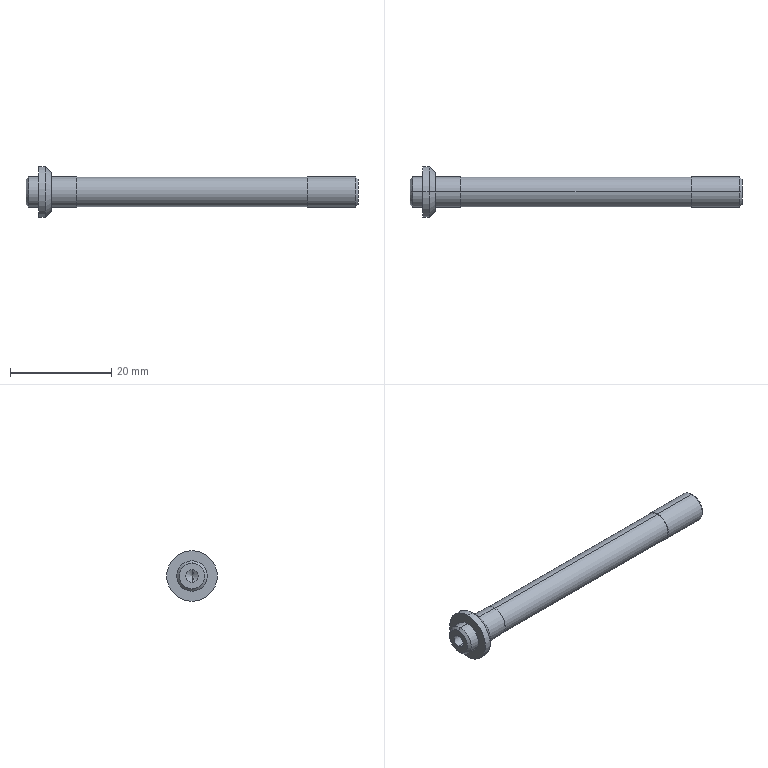Part | SolidWorks | features Chamfer 2, HoleWzd 1, Revolution 1 | 1 solid | 26 faces | box 65.5 x 10 x 10 mm | volume 1830 mm3 | cylinder 12 | cone 8 | plane 6 | commonest cylinder face diameters 6 x6 2.5 x2 5.8 x2 10 x2
STEP:
#1=CARTESIAN_POINT('',(65.5,0.,-2.5));
#2=VERTEX_POINT('',#1);
#3=CARTESIAN_POINT('',(65.5,0.,2.5));
#4=VERTEX_POINT('',#3);
#5=CARTESIAN_POINT('',(65.5,0.,0.));
#6=DIRECTION('',(1.,0.,0.));
#7=DIRECTION('',(0.,0.,1.));
#8=AXIS2_PLACEMENT_3D('',#5,#6,#7);
#9=CIRCLE('',#8,2.5);
#10=EDGE_CURVE('',#2,#4,#9,.T.);
#11=ORIENTED_EDGE('',*,*,#10,.F.);
#12=CARTESIAN_POINT('',(65.,0.,-3.));
#13=VERTEX_POINT('',#12);
#14=CARTESIAN_POINT('',(65.,0.,-3.));
#15=DIRECTION('',(-0.7071,0.,-0.7071));
#16=VECTOR('',#15,1000.);
#17=LINE('',#14,#16);
#18=EDGE_CURVE('',#2,#13,#17,.T.);
#19=ORIENTED_EDGE('',*,*,#18,.T.);
#20=CARTESIAN_POINT('',(65.,0.,3.));
#21=VERTEX_POINT('',#20);
#22=CARTESIAN_POINT('',(65.,0.,0.));
#23=DIRECTION('',(-1.,0.,0.));
#24=DIRECTION('',(0.,0.,1.));
#25=AXIS2_PLACEMENT_3D('',#22,#23,#24);
#26=CIRCLE('',#25,3.);
#27=EDGE_CURVE('',#21,#13,#26,.T.);
#28=ORIENTED_EDGE('',*,*,#27,.F.);
#29=CARTESIAN_POINT('',(65.,0.,3.));
#30=DIRECTION('',(-0.7071,0.,0.7071));
#31=VECTOR('',#30,1000.);
#32=LINE('',#29,#31);
#33=EDGE_CURVE('',#4,#21,#32,.T.);
#34=ORIENTED_EDGE('',*,*,#33,.F.);
#35=EDGE_LOOP('',(#11,#19,#28,#34));
#36=FACE_OUTER_BOUND('',#35,.T.);
#37=CARTESIAN_POINT('',(65.,0.,0.));
#38=DIRECTION('',(-1.,0.,0.));
#39=DIRECTION('',(0.,0.,1.));
#40=AXIS2_PLACEMENT_3D('',#37,#38,#39);
#41=CONICAL_SURFACE('',#40,3.,0.7854);
#42=ADVANCED_FACE('',(#36),#41,.T.);
#43=CARTESIAN_POINT('',(0.,0.,2.5));
#44=VERTEX_POINT('',#43);
#45=CARTESIAN_POINT('',(0.,0.,-2.5));
#46=VERTEX_POINT('',#45);
#47=CARTESIAN_POINT('',(0.,0.,0.));
#48=DIRECTION('',(-1.,0.,0.));
#49=DIRECTION('',(0.,0.,-1.));
#50=AXIS2_PLACEMENT_3D('',#47,#48,#49);
#51=CIRCLE('',#50,2.5);
#52=EDGE_CURVE('',#44,#46,#51,.T.);
#53=ORIENTED_EDGE('',*,*,#52,.F.);
#54=CARTESIAN_POINT('',(0.5,0.,3.));
#55=VERTEX_POINT('',#54);
#56=CARTESIAN_POINT('',(0.,0.,2.5));
#57=DIRECTION('',(0.7071,0.,0.7071));
#58=VECTOR('',#57,1000.);
#59=LINE('',#56,#58);
#60=EDGE_CURVE('',#44,#55,#59,.T.);
#61=ORIENTED_EDGE('',*,*,#60,.T.);
#62=CARTESIAN_POINT('',(0.5,0.,-3.));
#63=VERTEX_POINT('',#62);
#64=CARTESIAN_POINT('',(0.5,0.,0.));
#65=DIRECTION('',(1.,0.,0.));
#66=DIRECTION('',(0.,0.,-1.));
#67=AXIS2_PLACEMENT_3D('',#64,#65,#66);
#68=CIRCLE('',#67,3.);
#69=EDGE_CURVE('',#63,#55,#68,.T.);
#70=ORIENTED_EDGE('',*,*,#69,.F.);
#71=CARTESIAN_POINT('',(0.,0.,-2.5));
#72=DIRECTION('',(0.7071,0.,-0.7071));
#73=VECTOR('',#72,1000.);
#74=LINE('',#71,#73);
#75=EDGE_CURVE('',#46,#63,#74,.T.);
#76=ORIENTED_EDGE('',*,*,#75,.F.);
#77=EDGE_LOOP('',(#53,#61,#70,#76));
#78=FACE_OUTER_BOUND('',#77,.T.);
#79=CARTESIAN_POINT('',(0.,0.,0.));
#80=DIRECTION('',(1.,0.,0.));
#81=DIRECTION('',(0.,0.,-1.));
#82=AXIS2_PLACEMENT_3D('',#79,#80,#81);
#83=CONICAL_SURFACE('',#82,2.5,0.7854);
#84=ADVANCED_FACE('',(#78),#83,.T.);
#85=CARTESIAN_POINT('',(7.5,0.,-1.25));
#86=VERTEX_POINT('',#85);
#87=CARTESIAN_POINT('',(7.5,0.,1.25));
#88=VERTEX_POINT('',#87);
#89=CARTESIAN_POINT('',(7.5,0.,0.));
#90=DIRECTION('',(-1.,0.,0.));
#91=DIRECTION('',(0.,0.,1.));
#92=AXIS2_PLACEMENT_3D('',#89,#90,#91);
#93=CIRCLE('',#92,1.25);
#94=EDGE_CURVE('',#86,#88,#93,.T.);
#95=ORIENTED_EDGE('',*,*,#94,.F.);
#96=CARTESIAN_POINT('',(0.,0.,-1.25));
#97=VERTEX_POINT('',#96);
#98=CARTESIAN_POINT('',(0.,0.,-1.25));
#99=DIRECTION('',(-1.,0.,0.));
#100=VECTOR('',#99,1000.);
#101=LINE('',#98,#100);
#102=EDGE_CURVE('',#86,#97,#101,.T.);
#103=ORIENTED_EDGE('',*,*,#102,.T.);
#104=CARTESIAN_POINT('',(0.,0.,1.25));
#105=VERTEX_POINT('',#104);
#106=CARTESIAN_POINT('',(0.,0.,0.));
#107=DIRECTION('',(-1.,0.,0.));
#108=DIRECTION('',(0.,0.,1.));
#109=AXIS2_PLACEMENT_3D('',#106,#107,#108);
#110=CIRCLE('',#109,1.25);
#111=EDGE_CURVE('',#97,#105,#110,.T.);
#112=ORIENTED_EDGE('',*,*,#111,.T.);
#113=CARTESIAN_POINT('',(0.,0.,1.25));
#114=DIRECTION('',(-1.,0.,0.));
#115=VECTOR('',#114,1000.);
#116=LINE('',#113,#115);
#117=EDGE_CURVE('',#88,#105,#116,.T.);
#118=ORIENTED_EDGE('',*,*,#117,.F.);
#119=EDGE_LOOP('',(#95,#103,#112,#118));
#120=FACE_OUTER_BOUND('',#119,.T.);
#121=CARTESIAN_POINT('',(0.,0.,0.));
#122=DIRECTION('',(-1.,0.,0.));
#123=DIRECTION('',(0.,0.,1.));
#124=AXIS2_PLACEMENT_3D('',#121,#122,#123);
#125=CYLINDRICAL_SURFACE('',#124,1.25);
#126=ADVANCED_FACE('',(#120),#125,.F.);
#127=CARTESIAN_POINT('',(8.251,0.,0.));
#128=VERTEX_POINT('',#127);
#129=CARTESIAN_POINT('',(7.5,0.,1.25));
#130=DIRECTION('',(-0.515,0.,0.8572));
#131=VECTOR('',#130,1000.);
#132=LINE('',#129,#131);
#133=EDGE_CURVE('',#128,#88,#132,.T.);
#134=ORIENTED_EDGE('',*,*,#133,.F.);
#135=CARTESIAN_POINT('',(7.5,0.,-1.25));
#136=DIRECTION('',(-0.515,0.,-0.8572));
#137=VECTOR('',#136,1000.);
#138=LINE('',#135,#137);
#139=EDGE_CURVE('',#128,#86,#138,.T.);
#140=ORIENTED_EDGE('',*,*,#139,.T.);
#141=ORIENTED_EDGE('',*,*,#94,.T.);
#142=EDGE_LOOP('',(#134,#140,#141));
#143=FACE_OUTER_BOUND('',#142,.T.);
#144=CARTESIAN_POINT('',(7.5,0.,0.));
#145=DIRECTION('',(-1.,0.,0.));
#146=DIRECTION('',(0.,0.,1.));
#147=AXIS2_PLACEMENT_3D('',#144,#145,#146);
#148=CONICAL_SURFACE('',#147,1.25,1.03);
#149=ADVANCED_FACE('',(#143),#148,.F.);
#150=CARTESIAN_POINT('',(5.,0.,-3.8));
#151=VERTEX_POINT('',#150);
#152=CARTESIAN_POINT('',(5.,0.,3.8));
#153=VERTEX_POINT('',#152);
#154=CARTESIAN_POINT('',(5.,0.,0.));
#155=DIRECTION('',(1.,0.,0.));
#156=DIRECTION('',(0.,0.,1.));
#157=AXIS2_PLACEMENT_3D('',#154,#155,#156);
#158=CIRCLE('',#157,3.8);
#159=EDGE_CURVE('',#151,#153,#158,.T.);
#160=ORIENTED_EDGE('',*,*,#159,.F.);
#161=CARTESIAN_POINT('',(3.8,0.,-5.));
#162=VERTEX_POINT('',#161);
#163=CARTESIAN_POINT('',(3.8,0.,-5.));
#164=DIRECTION('',(-0.7071,0.,-0.7071));
#165=VECTOR('',#164,1000.);
#166=LINE('',#163,#165);
#167=EDGE_CURVE('',#151,#162,#166,.T.);
#168=ORIENTED_EDGE('',*,*,#167,.T.);
#169=CARTESIAN_POINT('',(3.8,0.,5.));
#170=VERTEX_POINT('',#169);
#171=CARTESIAN_POINT('',(3.8,0.,0.));
#172=DIRECTION('',(-1.,0.,0.));
#173=DIRECTION('',(0.,0.,1.));
#174=AXIS2_PLACEMENT_3D('',#171,#172,#173);
#175=CIRCLE('',#174,5.);
#176=EDGE_CURVE('',#170,#162,#175,.T.);
#177=ORIENTED_EDGE('',*,*,#176,.F.);
#178=CARTESIAN_POINT('',(3.8,0.,5.));
#179=DIRECTION('',(-0.7071,0.,0.7071));
#180=VECTOR('',#179,1000.);
#181=LINE('',#178,#180);
#182=EDGE_CURVE('',#153,#170,#181,.T.);
#183=ORIENTED_EDGE('',*,*,#182,.F.);
#184=EDGE_LOOP('',(#160,#168,#177,#183));
#185=FACE_OUTER_BOUND('',#184,.T.);
#186=CARTESIAN_POINT('',(3.8,0.,0.));
#187=DIRECTION('',(-1.,0.,0.));
#188=DIRECTION('',(0.,0.,1.));
#189=AXIS2_PLACEMENT_3D('',#186,#187,#188);
#190=CONICAL_SURFACE('',#189,5.,0.7854);
#191=ADVANCED_FACE('',(#185),#190,.T.);
#192=ORIENTED_EDGE('',*,*,#27,.T.);
#193=CARTESIAN_POINT('',(55.5,0.,-3.));
#194=VERTEX_POINT('',#193);
#195=CARTESIAN_POINT('',(0.,0.,-3.));
#196=DIRECTION('',(-1.,0.,0.));
#197=VECTOR('',#196,1000.);
#198=LINE('',#195,#197);
#199=EDGE_CURVE('',#13,#194,#198,.T.);
#200=ORIENTED_EDGE('',*,*,#199,.T.);
#201=CARTESIAN_POINT('',(55.5,0.,3.));
#202=VERTEX_POINT('',#201);
#203=CARTESIAN_POINT('',(55.5,0.,0.));
#204=DIRECTION('',(-1.,0.,0.));
#205=DIRECTION('',(0.,0.,1.));
#206=AXIS2_PLACEMENT_3D('',#203,#204,#205);
#207=CIRCLE('',#206,3.);
#208=EDGE_CURVE('',#202,#194,#207,.T.);
#209=ORIENTED_EDGE('',*,*,#208,.F.);
#210=CARTESIAN_POINT('',(0.,0.,3.));
#211=DIRECTION('',(-1.,0.,0.));
#212=VECTOR('',#211,1000.);
#213=LINE('',#210,#212);
#214=EDGE_CURVE('',#21,#202,#213,.T.);
#215=ORIENTED_EDGE('',*,*,#214,.F.);
#216=EDGE_LOOP('',(#192,#200,#209,#215));
#217=FACE_OUTER_BOUND('',#216,.T.);
#218=CARTESIAN_POINT('',(0.,0.,0.));
#219=DIRECTION('',(-1.,0.,0.));
#220=DIRECTION('',(0.,0.,1.));
#221=AXIS2_PLACEMENT_3D('',#218,#219,#220);
#222=CYLINDRICAL_SURFACE('',#221,3.);
#223=ADVANCED_FACE('',(#217),#222,.T.);
#224=CARTESIAN_POINT('',(55.5,0.,2.9));
#225=VERTEX_POINT('',#224);
#226=CARTESIAN_POINT('',(55.5,0.,-2.9));
#227=VERTEX_POINT('',#226);
#228=CARTESIAN_POINT('',(55.5,0.,0.));
#229=DIRECTION('',(-1.,0.,0.));
#230=DIRECTION('',(0.,0.,1.));
#231=AXIS2_PLACEMENT_3D('',#228,#229,#230);
#232=CIRCLE('',#231,2.9);
#233=EDGE_CURVE('',#225,#227,#232,.T.);
#234=ORIENTED_EDGE('',*,*,#233,.T.);
#235=CARTESIAN_POINT('',(10.,0.,-2.9));
#236=VERTEX_POINT('',#235);
#237=CARTESIAN_POINT('',(0.,0.,-2.9));
#238=DIRECTION('',(-1.,0.,0.));
#239=VECTOR('',#238,1000.);
#240=LINE('',#237,#239);
#241=EDGE_CURVE('',#227,#236,#240,.T.);
#242=ORIENTED_EDGE('',*,*,#241,.T.);
#243=CARTESIAN_POINT('',(10.,0.,2.9));
#244=VERTEX_POINT('',#243);
#245=CARTESIAN_POINT('',(10.,0.,0.));
#246=DIRECTION('',(-1.,0.,0.));
#247=DIRECTION('',(0.,0.,1.));
#248=AXIS2_PLACEMENT_3D('',#245,#246,#247);
#249=CIRCLE('',#248,2.9);
#250=EDGE_CURVE('',#244,#236,#249,.T.);
#251=ORIENTED_EDGE('',*,*,#250,.F.);
#252=CARTESIAN_POINT('',(0.,0.,2.9));
#253=DIRECTION('',(-1.,0.,0.));
#254=VECTOR('',#253,1000.);
#255=LINE('',#252,#254);
#256=EDGE_CURVE('',#225,#244,#255,.T.);
#257=ORIENTED_EDGE('',*,*,#256,.F.);
#258=EDGE_LOOP('',(#234,#242,#251,#257));
#259=FACE_OUTER_BOUND('',#258,.T.);
#260=CARTESIAN_POINT('',(0.,0.,0.));
#261=DIRECTION('',(-1.,0.,0.));
#262=DIRECTION('',(0.,0.,1.));
#263=AXIS2_PLACEMENT_3D('',#260,#261,#262);
#264=CYLINDRICAL_SURFACE('',#263,2.9);
#265=ADVANCED_FACE('',(#259),#264,.T.);
#266=CARTESIAN_POINT('',(10.,0.,3.));
#267=VERTEX_POINT('',#266);
#268=CARTESIAN_POINT('',(10.,0.,-3.));
#269=VERTEX_POINT('',#268);
#270=CARTESIAN_POINT('',(10.,0.,0.));
#271=DIRECTION('',(-1.,0.,0.));
#272=DIRECTION('',(0.,0.,1.));
#273=AXIS2_PLACEMENT_3D('',#270,#271,#272);
#274=CIRCLE('',#273,3.);
#275=EDGE_CURVE('',#267,#269,#274,.T.);
#276=ORIENTED_EDGE('',*,*,#275,.T.);
#277=CARTESIAN_POINT('',(5.,0.,-3.));
#278=VERTEX_POINT('',#277);
#279=CARTESIAN_POINT('',(0.,0.,-3.));
#280=DIRECTION('',(-1.,0.,0.));
#281=VECTOR('',#280,1000.);
#282=LINE('',#279,#281);
#283=EDGE_CURVE('',#269,#278,#282,.T.);
#284=ORIENTED_EDGE('',*,*,#283,.T.);
#285=CARTESIAN_POINT('',(5.,0.,3.));
#286=VERTEX_POINT('',#285);
#287=CARTESIAN_POINT('',(5.,0.,0.));
#288=DIRECTION('',(-1.,0.,0.));
#289=DIRECTION('',(0.,0.,1.));
#290=AXIS2_PLACEMENT_3D('',#287,#288,#289);
#291=CIRCLE('',#290,3.);
#292=EDGE_CURVE('',#286,#278,#291,.T.);
#293=ORIENTED_EDGE('',*,*,#292,.F.);
#294=CARTESIAN_POINT('',(0.,0.,3.));
#295=DIRECTION('',(-1.,0.,0.));
#296=VECTOR('',#295,1000.);
#297=LINE('',#294,#296);
#298=EDGE_CURVE('',#267,#286,#297,.T.);
#299=ORIENTED_EDGE('',*,*,#298,.F.);
#300=EDGE_LOOP('',(#276,#284,#293,#299));
#301=FACE_OUTER_BOUND('',#300,.T.);
#302=CARTESIAN_POINT('',(0.,0.,0.));
#303=DIRECTION('',(-1.,0.,0.));
#304=DIRECTION('',(0.,0.,1.));
#305=AXIS2_PLACEMENT_3D('',#302,#303,#304);
#306=CYLINDRICAL_SURFACE('',#305,3.);
#307=ADVANCED_FACE('',(#301),#306,.T.);
#308=ORIENTED_EDGE('',*,*,#176,.T.);
#309=CARTESIAN_POINT('',(2.5,0.,-5.));
#310=VERTEX_POINT('',#309);
#311=CARTESIAN_POINT('',(0.,0.,-5.));
#312=DIRECTION('',(-1.,0.,0.));
#313=VECTOR('',#312,1000.);
#314=LINE('',#311,#313);
#315=EDGE_CURVE('',#162,#310,#314,.T.);
#316=ORIENTED_EDGE('',*,*,#315,.T.);
#317=CARTESIAN_POINT('',(2.5,0.,5.));
#318=VERTEX_POINT('',#317);
#319=CARTESIAN_POINT('',(2.5,0.,0.));
#320=DIRECTION('',(-1.,0.,0.));
#321=DIRECTION('',(0.,0.,1.));
#322=AXIS2_PLACEMENT_3D('',#319,#320,#321);
#323=CIRCLE('',#322,5.);
#324=EDGE_CURVE('',#318,#310,#323,.T.);
#325=ORIENTED_EDGE('',*,*,#324,.F.);
#326=CARTESIAN_POINT('',(0.,0.,5.));
#327=DIRECTION('',(-1.,0.,0.));
#328=VECTOR('',#327,1000.);
#329=LINE('',#326,#328);
#330=EDGE_CURVE('',#170,#318,#329,.T.);
#331=ORIENTED_EDGE('',*,*,#330,.F.);
#332=EDGE_LOOP('',(#308,#316,#325,#331));
#333=FACE_OUTER_BOUND('',#332,.T.);
#334=CARTESIAN_POINT('',(0.,0.,0.));
#335=DIRECTION('',(-1.,0.,0.));
#336=DIRECTION('',(0.,0.,1.));
#337=AXIS2_PLACEMENT_3D('',#334,#335,#336);
#338=CYLINDRICAL_SURFACE('',#337,5.);
#339=ADVANCED_FACE('',(#333),#338,.T.);
#340=CARTESIAN_POINT('',(2.5,0.,3.));
#341=VERTEX_POINT('',#340);
#342=CARTESIAN_POINT('',(2.5,0.,-3.));
#343=VERTEX_POINT('',#342);
#344=CARTESIAN_POINT('',(2.5,0.,0.));
#345=DIRECTION('',(-1.,0.,0.));
#346=DIRECTION('',(0.,0.,1.));
#347=AXIS2_PLACEMENT_3D('',#344,#345,#346);
#348=CIRCLE('',#347,3.);
#349=EDGE_CURVE('',#341,#343,#348,.T.);
#350=ORIENTED_EDGE('',*,*,#349,.T.);
#351=CARTESIAN_POINT('',(0.,0.,-3.));
#352=DIRECTION('',(-1.,0.,0.));
#353=VECTOR('',#352,1000.);
#354=LINE('',#351,#353);
#355=EDGE_CURVE('',#343,#63,#354,.T.);
#356=ORIENTED_EDGE('',*,*,#355,.T.);
#357=ORIENTED_EDGE('',*,*,#69,.T.);
#358=CARTESIAN_POINT('',(0.,0.,3.));
#359=DIRECTION('',(-1.,0.,0.));
#360=VECTOR('',#359,1000.);
#361=LINE('',#358,#360);
#362=EDGE_CURVE('',#341,#55,#361,.T.);
#363=ORIENTED_EDGE('',*,*,#362,.F.);
#364=EDGE_LOOP('',(#350,#356,#357,#363));
#365=FACE_OUTER_BOUND('',#364,.T.);
#366=CARTESIAN_POINT('',(0.,0.,0.));
#367=DIRECTION('',(-1.,0.,0.));
#368=DIRECTION('',(0.,0.,1.));
#369=AXIS2_PLACEMENT_3D('',#366,#367,#368);
#370=CYLINDRICAL_SURFACE('',#369,3.);
#371=ADVANCED_FACE('',(#365),#370,.T.);
#372=CARTESIAN_POINT('',(0.,0.,0.));
#373=DIRECTION('',(-1.,0.,0.));
#374=DIRECTION('',(0.,0.,-1.));
#375=AXIS2_PLACEMENT_3D('',#372,#373,#374);
#376=CIRCLE('',#375,2.5);
#377=EDGE_CURVE('',#46,#44,#376,.T.);
#378=ORIENTED_EDGE('',*,*,#377,.T.);
#379=ORIENTED_EDGE('',*,*,#52,.T.);
#380=EDGE_LOOP('',(#378,#379));
#381=FACE_OUTER_BOUND('',#380,.T.);
#382=CARTESIAN_POINT('',(0.,0.,0.));
#383=DIRECTION('',(-1.,0.,0.));
#384=DIRECTION('',(0.,0.,1.));
#385=AXIS2_PLACEMENT_3D('',#382,#383,#384);
#386=CIRCLE('',#385,1.25);
#387=EDGE_CURVE('',#105,#97,#386,.T.);
#388=ORIENTED_EDGE('',*,*,#387,.F.);
#389=ORIENTED_EDGE('',*,*,#111,.F.);
#390=EDGE_LOOP('',(#388,#389));
#391=FACE_BOUND('',#390,.T.);
#392=CARTESIAN_POINT('',(0.,0.,0.));
#393=DIRECTION('',(1.,0.,0.));
#394=DIRECTION('',(0.,0.,-1.));
#395=AXIS2_PLACEMENT_3D('',#392,#393,#394);
#396=PLANE('',#395);
#397=ADVANCED_FACE('',(#381,#391),#396,.F.);
#398=ORIENTED_EDGE('',*,*,#355,.F.);
#399=CARTESIAN_POINT('',(2.5,0.,0.));
#400=DIRECTION('',(-1.,0.,0.));
#401=DIRECTION('',(0.,0.,1.));
#402=AXIS2_PLACEMENT_3D('',#399,#400,#401);
#403=CIRCLE('',#402,3.);
#404=EDGE_CURVE('',#343,#341,#403,.T.);
#405=ORIENTED_EDGE('',*,*,#404,.T.);
#406=ORIENTED_EDGE('',*,*,#362,.T.);
#407=CARTESIAN_POINT('',(0.5,0.,0.));
#408=DIRECTION('',(1.,0.,0.));
#409=DIRECTION('',(0.,0.,-1.));
#410=AXIS2_PLACEMENT_3D('',#407,#408,#409);
#411=CIRCLE('',#410,3.);
#412=EDGE_CURVE('',#55,#63,#411,.T.);
#413=ORIENTED_EDGE('',*,*,#412,.T.);
#414=EDGE_LOOP('',(#398,#405,#406,#413));
#415=FACE_OUTER_BOUND('',#414,.T.);
#416=CARTESIAN_POINT('',(0.,0.,0.));
#417=DIRECTION('',(-1.,0.,0.));
#418=DIRECTION('',(0.,0.,1.));
#419=AXIS2_PLACEMENT_3D('',#416,#417,#418);
#420=CYLINDRICAL_SURFACE('',#419,3.);
#421=ADVANCED_FACE('',(#415),#420,.T.);
#422=ORIENTED_EDGE('',*,*,#349,.F.);
#423=ORIENTED_EDGE('',*,*,#404,.F.);
#424=EDGE_LOOP('',(#422,#423));
#425=FACE_BOUND('',#424,.T.);
#426=ORIENTED_EDGE('',*,*,#324,.T.);
#427=CARTESIAN_POINT('',(2.5,0.,0.));
#428=DIRECTION('',(-1.,0.,0.));
#429=DIRECTION('',(0.,0.,1.));
#430=AXIS2_PLACEMENT_3D('',#427,#428,#429);
#431=CIRCLE('',#430,5.);
#432=EDGE_CURVE('',#310,#318,#431,.T.);
#433=ORIENTED_EDGE('',*,*,#432,.T.);
#434=EDGE_LOOP('',(#426,#433));
#435=FACE_OUTER_BOUND('',#434,.T.);
#436=CARTESIAN_POINT('',(2.5,3.,0.));
#437=DIRECTION('',(1.,0.,0.));
#438=DIRECTION('',(0.,0.,-1.));
#439=AXIS2_PLACEMENT_3D('',#436,#437,#438);
#440=PLANE('',#439);
#441=ADVANCED_FACE('',(#425,#435),#440,.F.);
#442=ORIENTED_EDGE('',*,*,#315,.F.);
#443=CARTESIAN_POINT('',(3.8,0.,0.));
#444=DIRECTION('',(-1.,0.,0.));
#445=DIRECTION('',(0.,0.,1.));
#446=AXIS2_PLACEMENT_3D('',#443,#444,#445);
#447=CIRCLE('',#446,5.);
#448=EDGE_CURVE('',#162,#170,#447,.T.);
#449=ORIENTED_EDGE('',*,*,#448,.T.);
#450=ORIENTED_EDGE('',*,*,#330,.T.);
#451=ORIENTED_EDGE('',*,*,#432,.F.);
#452=EDGE_LOOP('',(#442,#449,#450,#451));
#453=FACE_OUTER_BOUND('',#452,.T.);
#454=CARTESIAN_POINT('',(0.,0.,0.));
#455=DIRECTION('',(-1.,0.,0.));
#456=DIRECTION('',(0.,0.,1.));
#457=AXIS2_PLACEMENT_3D('',#454,#455,#456);
#458=CYLINDRICAL_SURFACE('',#457,5.);
#459=ADVANCED_FACE('',(#453),#458,.T.);
#460=CARTESIAN_POINT('',(5.,0.,0.));
#461=DIRECTION('',(1.,0.,0.));
#462=DIRECTION('',(0.,0.,1.));
#463=AXIS2_PLACEMENT_3D('',#460,#461,#462);
#464=CIRCLE('',#463,3.8);
#465=EDGE_CURVE('',#153,#151,#464,.T.);
#466=ORIENTED_EDGE('',*,*,#465,.T.);
#467=ORIENTED_EDGE('',*,*,#159,.T.);
#468=EDGE_LOOP('',(#466,#467));
#469=FACE_OUTER_BOUND('',#468,.T.);
#470=ORIENTED_EDGE('',*,*,#292,.T.);
#471=CARTESIAN_POINT('',(5.,0.,0.));
#472=DIRECTION('',(-1.,0.,0.));
#473=DIRECTION('',(0.,0.,1.));
#474=AXIS2_PLACEMENT_3D('',#471,#472,#473);
#475=CIRCLE('',#474,3.);
#476=EDGE_CURVE('',#278,#286,#475,.T.);
#477=ORIENTED_EDGE('',*,*,#476,.T.);
#478=EDGE_LOOP('',(#470,#477));
#479=FACE_BOUND('',#478,.T.);
#480=CARTESIAN_POINT('',(5.,5.,0.));
#481=DIRECTION('',(-1.,0.,0.));
#482=DIRECTION('',(0.,0.,1.));
#483=AXIS2_PLACEMENT_3D('',#480,#481,#482);
#484=PLANE('',#483);
#485=ADVANCED_FACE('',(#469,#479),#484,.F.);
#486=ORIENTED_EDGE('',*,*,#283,.F.);
#487=CARTESIAN_POINT('',(10.,0.,0.));
#488=DIRECTION('',(-1.,0.,0.));
#489=DIRECTION('',(0.,0.,1.));
#490=AXIS2_PLACEMENT_3D('',#487,#488,#489);
#491=CIRCLE('',#490,3.);
#492=EDGE_CURVE('',#269,#267,#491,.T.);
#493=ORIENTED_EDGE('',*,*,#492,.T.);
#494=ORIENTED_EDGE('',*,*,#298,.T.);
#495=ORIENTED_EDGE('',*,*,#476,.F.);
#496=EDGE_LOOP('',(#486,#493,#494,#495));
#497=FACE_OUTER_BOUND('',#496,.T.);
#498=CARTESIAN_POINT('',(0.,0.,0.));
#499=DIRECTION('',(-1.,0.,0.));
#500=DIRECTION('',(0.,0.,1.));
#501=AXIS2_PLACEMENT_3D('',#498,#499,#500);
#502=CYLINDRICAL_SURFACE('',#501,3.);
#503=ADVANCED_FACE('',(#497),#502,.T.);
#504=ORIENTED_EDGE('',*,*,#275,.F.);
#505=ORIENTED_EDGE('',*,*,#492,.F.);
#506=EDGE_LOOP('',(#504,#505));
#507=FACE_OUTER_BOUND('',#506,.T.);
#508=ORIENTED_EDGE('',*,*,#250,.T.);
#509=CARTESIAN_POINT('',(10.,0.,0.));
#510=DIRECTION('',(-1.,0.,0.));
#511=DIRECTION('',(0.,0.,1.));
#512=AXIS2_PLACEMENT_3D('',#509,#510,#511);
#513=CIRCLE('',#512,2.9);
#514=EDGE_CURVE('',#236,#244,#513,.T.);
#515=ORIENTED_EDGE('',*,*,#514,.T.);
#516=EDGE_LOOP('',(#508,#515));
#517=FACE_BOUND('',#516,.T.);
#518=CARTESIAN_POINT('',(10.,3.,0.));
#519=DIRECTION('',(-1.,0.,0.));
#520=DIRECTION('',(0.,0.,1.));
#521=AXIS2_PLACEMENT_3D('',#518,#519,#520);
#522=PLANE('',#521);
#523=ADVANCED_FACE('',(#507,#517),#522,.F.);
#524=ORIENTED_EDGE('',*,*,#241,.F.);
#525=CARTESIAN_POINT('',(55.5,0.,0.));
#526=DIRECTION('',(-1.,0.,0.));
#527=DIRECTION('',(0.,0.,1.));
#528=AXIS2_PLACEMENT_3D('',#525,#526,#527);
#529=CIRCLE('',#528,2.9);
#530=EDGE_CURVE('',#227,#225,#529,.T.);
#531=ORIENTED_EDGE('',*,*,#530,.T.);
#532=ORIENTED_EDGE('',*,*,#256,.T.);
#533=ORIENTED_EDGE('',*,*,#514,.F.);
#534=EDGE_LOOP('',(#524,#531,#532,#533));
#535=FACE_OUTER_BOUND('',#534,.T.);
#536=CARTESIAN_POINT('',(0.,0.,0.));
#537=DIRECTION('',(-1.,0.,0.));
#538=DIRECTION('',(0.,0.,1.));
#539=AXIS2_PLACEMENT_3D('',#536,#537,#538);
#540=CYLINDRICAL_SURFACE('',#539,2.9);
#541=ADVANCED_FACE('',(#535),#540,.T.);
#542=ORIENTED_EDGE('',*,*,#233,.F.);
#543=ORIENTED_EDGE('',*,*,#530,.F.);
#544=EDGE_LOOP('',(#542,#543));
#545=FACE_BOUND('',#544,.T.);
#546=ORIENTED_EDGE('',*,*,#208,.T.);
#547=CARTESIAN_POINT('',(55.5,0.,0.));
#548=DIRECTION('',(-1.,0.,0.));
#549=DIRECTION('',(0.,0.,1.));
#550=AXIS2_PLACEMENT_3D('',#547,#548,#549);
#551=CIRCLE('',#550,3.);
#552=EDGE_CURVE('',#194,#202,#551,.T.);
#553=ORIENTED_EDGE('',*,*,#552,.T.);
#554=EDGE_LOOP('',(#546,#553));
#555=FACE_OUTER_BOUND('',#554,.T.);
#556=CARTESIAN_POINT('',(55.5,2.9,0.));
#557=DIRECTION('',(1.,0.,0.));
#558=DIRECTION('',(0.,0.,-1.));
#559=AXIS2_PLACEMENT_3D('',#556,#557,#558);
#560=PLANE('',#559);
#561=ADVANCED_FACE('',(#545,#555),#560,.F.);
#562=ORIENTED_EDGE('',*,*,#199,.F.);
#563=CARTESIAN_POINT('',(65.,0.,0.));
#564=DIRECTION('',(-1.,0.,0.));
#565=DIRECTION('',(0.,0.,1.));
#566=AXIS2_PLACEMENT_3D('',#563,#564,#565);
#567=CIRCLE('',#566,3.);
#568=EDGE_CURVE('',#13,#21,#567,.T.);
#569=ORIENTED_EDGE('',*,*,#568,.T.);
#570=ORIENTED_EDGE('',*,*,#214,.T.);
#571=ORIENTED_EDGE('',*,*,#552,.F.);
#572=EDGE_LOOP('',(#562,#569,#570,#571));
#573=FACE_OUTER_BOUND('',#572,.T.);
#574=CARTESIAN_POINT('',(0.,0.,0.));
#575=DIRECTION('',(-1.,0.,0.));
#576=DIRECTION('',(0.,0.,1.));
#577=AXIS2_PLACEMENT_3D('',#574,#575,#576);
#578=CYLINDRICAL_SURFACE('',#577,3.);
#579=ADVANCED_FACE('',(#573),#578,.T.);
#580=CARTESIAN_POINT('',(65.5,0.,0.));
#581=DIRECTION('',(1.,0.,0.));
#582=DIRECTION('',(0.,0.,1.));
#583=AXIS2_PLACEMENT_3D('',#580,#581,#582);
#584=CIRCLE('',#583,2.5);
#585=EDGE_CURVE('',#4,#2,#584,.T.);
#586=ORIENTED_EDGE('',*,*,#585,.T.);
#587=ORIENTED_EDGE('',*,*,#10,.T.);
#588=EDGE_LOOP('',(#586,#587));
#589=FACE_OUTER_BOUND('',#588,.T.);
#590=CARTESIAN_POINT('',(65.5,3.,0.));
#591=DIRECTION('',(-1.,0.,0.));
#592=DIRECTION('',(0.,0.,1.));
#593=AXIS2_PLACEMENT_3D('',#590,#591,#592);
#594=PLANE('',#593);
#595=ADVANCED_FACE('',(#589),#594,.F.);
#596=ORIENTED_EDGE('',*,*,#167,.F.);
#597=ORIENTED_EDGE('',*,*,#465,.F.);
#598=ORIENTED_EDGE('',*,*,#182,.T.);
#599=ORIENTED_EDGE('',*,*,#448,.F.);
#600=EDGE_LOOP('',(#596,#597,#598,#599));
#601=FACE_OUTER_BOUND('',#600,.T.);
#602=CARTESIAN_POINT('',(3.8,0.,0.));
#603=DIRECTION('',(-1.,0.,0.));
#604=DIRECTION('',(0.,0.,1.));
#605=AXIS2_PLACEMENT_3D('',#602,#603,#604);
#606=CONICAL_SURFACE('',#605,5.,0.7854);
#607=ADVANCED_FACE('',(#601),#606,.T.);
#608=ORIENTED_EDGE('',*,*,#139,.F.);
#609=ORIENTED_EDGE('',*,*,#133,.T.);
#610=CARTESIAN_POINT('',(7.5,0.,0.));
#611=DIRECTION('',(-1.,0.,0.));
#612=DIRECTION('',(0.,0.,1.));
#613=AXIS2_PLACEMENT_3D('',#610,#611,#612);
#614=CIRCLE('',#613,1.25);
#615=EDGE_CURVE('',#88,#86,#614,.T.);
#616=ORIENTED_EDGE('',*,*,#615,.T.);
#617=EDGE_LOOP('',(#608,#609,#616));
#618=FACE_OUTER_BOUND('',#617,.T.);
#619=CARTESIAN_POINT('',(7.5,0.,0.));
#620=DIRECTION('',(-1.,0.,0.));
#621=DIRECTION('',(0.,0.,1.));
#622=AXIS2_PLACEMENT_3D('',#619,#620,#621);
#623=CONICAL_SURFACE('',#622,1.25,1.03);
#624=ADVANCED_FACE('',(#618),#623,.F.);
#625=ORIENTED_EDGE('',*,*,#102,.F.);
#626=ORIENTED_EDGE('',*,*,#615,.F.);
#627=ORIENTED_EDGE('',*,*,#117,.T.);
#628=ORIENTED_EDGE('',*,*,#387,.T.);
#629=EDGE_LOOP('',(#625,#626,#627,#628));
#630=FACE_OUTER_BOUND('',#629,.T.);
#631=CARTESIAN_POINT('',(0.,0.,0.));
#632=DIRECTION('',(-1.,0.,0.));
#633=DIRECTION('',(0.,0.,1.));
#634=AXIS2_PLACEMENT_3D('',#631,#632,#633);
#635=CYLINDRICAL_SURFACE('',#634,1.25);
#636=ADVANCED_FACE('',(#630),#635,.F.);
#637=ORIENTED_EDGE('',*,*,#60,.F.);
#638=ORIENTED_EDGE('',*,*,#377,.F.);
#639=ORIENTED_EDGE('',*,*,#75,.T.);
#640=ORIENTED_EDGE('',*,*,#412,.F.);
#641=EDGE_LOOP('',(#637,#638,#639,#640));
#642=FACE_OUTER_BOUND('',#641,.T.);
#643=CARTESIAN_POINT('',(0.,0.,0.));
#644=DIRECTION('',(1.,0.,0.));
#645=DIRECTION('',(0.,0.,-1.));
#646=AXIS2_PLACEMENT_3D('',#643,#644,#645);
#647=CONICAL_SURFACE('',#646,2.5,0.7854);
#648=ADVANCED_FACE('',(#642),#647,.T.);
#649=ORIENTED_EDGE('',*,*,#18,.F.);
#650=ORIENTED_EDGE('',*,*,#585,.F.);
#651=ORIENTED_EDGE('',*,*,#33,.T.);
#652=ORIENTED_EDGE('',*,*,#568,.F.);
#653=EDGE_LOOP('',(#649,#650,#651,#652));
#654=FACE_OUTER_BOUND('',#653,.T.);
#655=CARTESIAN_POINT('',(65.,0.,0.));
#656=DIRECTION('',(-1.,0.,0.));
#657=DIRECTION('',(0.,0.,1.));
#658=AXIS2_PLACEMENT_3D('',#655,#656,#657);
#659=CONICAL_SURFACE('',#658,3.,0.7854);
#660=ADVANCED_FACE('',(#654),#659,.T.);
#661=CLOSED_SHELL('',(#42,#84,#126,#149,#191,#223,#265,#307,#339,#371,#397,#421,#441,#459,#485,#503,#523,#541,#561,#579,#595,#607,#624,#636,#648,#660));
#662=MANIFOLD_SOLID_BREP('',#661);
#663=CARTESIAN_POINT('',(0.,0.,0.));
#664=DIRECTION('',(0.,0.,1.));
#665=DIRECTION('',(1.,0.,0.));
#666=AXIS2_PLACEMENT_3D('',#663,#664,#665);
#667=(LENGTH_UNIT()NAMED_UNIT(*)SI_UNIT(.MILLI.,.METRE.));
#668=UNCERTAINTY_MEASURE_WITH_UNIT(LENGTH_MEASURE(0.00001),#667,'','');
#669=(NAMED_UNIT(*)PLANE_ANGLE_UNIT()SI_UNIT($,.RADIAN.));
#670=(NAMED_UNIT(*)SI_UNIT($,.STERADIAN.)SOLID_ANGLE_UNIT());
#671=(GEOMETRIC_REPRESENTATION_CONTEXT(3)GLOBAL_UNCERTAINTY_ASSIGNED_CONTEXT((#668))GLOBAL_UNIT_ASSIGNED_CONTEXT((#667,#669,#670))REPRESENTATION_CONTEXT('',''));
#672=ADVANCED_BREP_SHAPE_REPRESENTATION('',(#662,#666),#671);